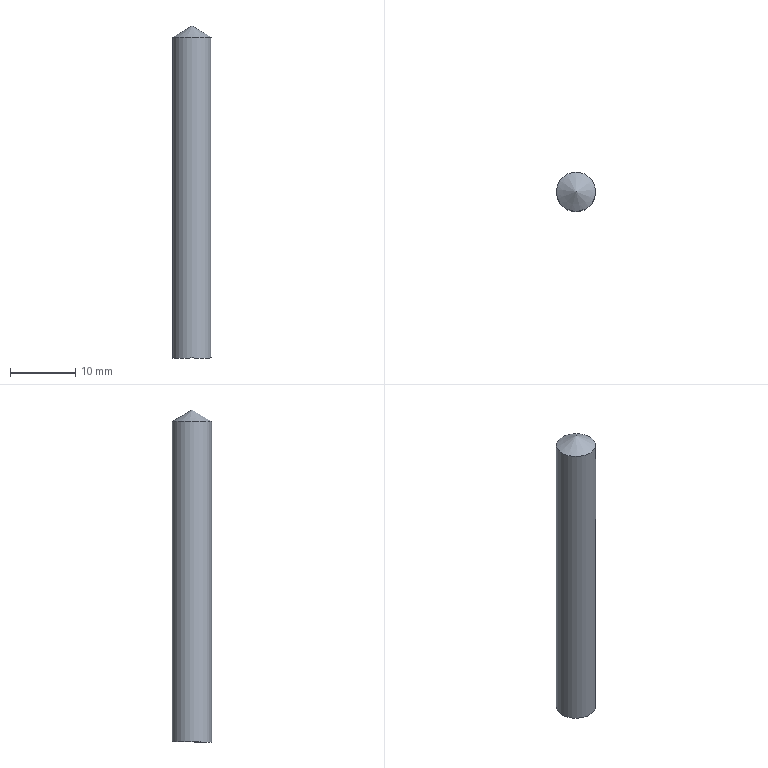Part | NX | features solid 2 | 1 solid | 3 faces | box 6 x 6 x 50.732 mm | volume 1402 mm3 | cylinder 1 | plane 1 | cone 1 | commonest cylinder face diameters 6 x1
STEP:
#1=CARTESIAN_POINT('',(-85.,-33.,104.));
#2=VERTEX_POINT('',#1);
#3=CARTESIAN_POINT('',(-85.,-30.,104.));
#4=DIRECTION('',(0.,0.,1.));
#5=DIRECTION('',(0.,-1.,0.));
#6=AXIS2_PLACEMENT_3D('',#3,#4,#5);
#7=CIRCLE('',#6,3.);
#8=EDGE_CURVE('',#2,#2,#7,.T.);
#9=ORIENTED_EDGE('',*,*,#8,.F.);
#10=EDGE_LOOP('',(#9));
#11=FACE_BOUND('',#10,.T.);
#12=CARTESIAN_POINT('',(-85.,-33.,55.));
#13=VERTEX_POINT('',#12);
#14=CARTESIAN_POINT('',(-85.,-30.,55.));
#15=DIRECTION('',(0.,0.,1.));
#16=DIRECTION('',(0.,-1.,0.));
#17=AXIS2_PLACEMENT_3D('',#14,#15,#16);
#18=CIRCLE('',#17,3.);
#19=EDGE_CURVE('',#13,#13,#18,.T.);
#20=ORIENTED_EDGE('',*,*,#19,.T.);
#21=EDGE_LOOP('',(#20));
#22=FACE_BOUND('',#21,.T.);
#23=CARTESIAN_POINT('',(-85.,-30.,100.));
#24=DIRECTION('',(0.,0.,-1.));
#25=DIRECTION('',(0.,1.,0.));
#26=AXIS2_PLACEMENT_3D('',#23,#24,#25);
#27=CYLINDRICAL_SURFACE('',#26,3.);
#28=ADVANCED_FACE('',(#11,#22),#27,.T.);
#29=ORIENTED_EDGE('',*,*,#19,.F.);
#30=EDGE_LOOP('',(#29));
#31=FACE_BOUND('',#30,.T.);
#32=CARTESIAN_POINT('',(-85.,-30.,55.));
#33=DIRECTION('',(0.,0.,1.));
#34=DIRECTION('',(0.,-1.,0.));
#35=AXIS2_PLACEMENT_3D('',#32,#33,#34);
#36=PLANE('',#35);
#37=ADVANCED_FACE('',(#31),#36,.F.);
#38=ORIENTED_EDGE('',*,*,#8,.T.);
#39=EDGE_LOOP('',(#38));
#40=FACE_BOUND('',#39,.T.);
#41=CARTESIAN_POINT('',(-85.,-30.,105.732));
#42=VERTEX_POINT('',#41);
#43=VERTEX_LOOP('',#42);
#44=FACE_BOUND('',#43,.T.);
#45=CARTESIAN_POINT('',(-85.,-30.,105.732));
#46=DIRECTION('',(0.,0.,-1.));
#47=DIRECTION('',(0.,1.,0.));
#48=AXIS2_PLACEMENT_3D('',#45,#46,#47);
#49=CONICAL_SURFACE('',#48,0.,1.047);
#50=ADVANCED_FACE('',(#40,#44),#49,.T.);
#51=CLOSED_SHELL('',(#28,#37,#50));
#52=MANIFOLD_SOLID_BREP('',#51);
#53=(LENGTH_UNIT()NAMED_UNIT(*)SI_UNIT(.MILLI.,.METRE.));
#54=UNCERTAINTY_MEASURE_WITH_UNIT(LENGTH_MEASURE(0.00001),#53,'','');
#55=(NAMED_UNIT(*)PLANE_ANGLE_UNIT()SI_UNIT($,.RADIAN.));
#56=(NAMED_UNIT(*)SI_UNIT($,.STERADIAN.)SOLID_ANGLE_UNIT());
#57=(GEOMETRIC_REPRESENTATION_CONTEXT(3)GLOBAL_UNCERTAINTY_ASSIGNED_CONTEXT((#54))GLOBAL_UNIT_ASSIGNED_CONTEXT((#53,#55,#56))REPRESENTATION_CONTEXT('',''));
#58=ADVANCED_BREP_SHAPE_REPRESENTATION('',(#52),#57);